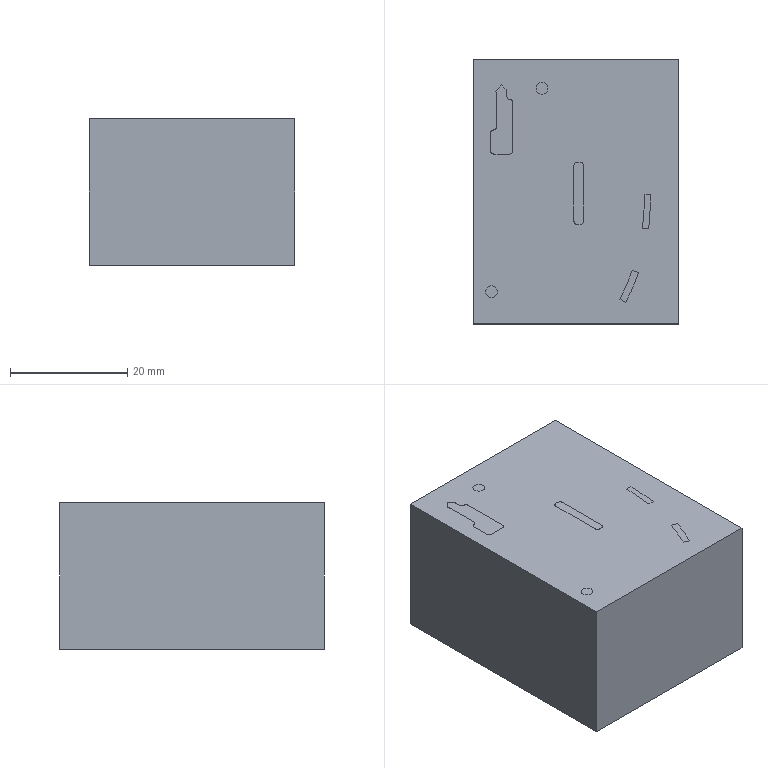Part | NX | features BREP 2 | 2 solids | 77 faces | box 35 x 45 x 25 mm | volume 74969 mm3 | plane 46 | cylinder 31 | commonest cylinder face diameters 1.1 x9 3.1 x9 0.9 x3 2 x2 67.073 x1 69.073 x1